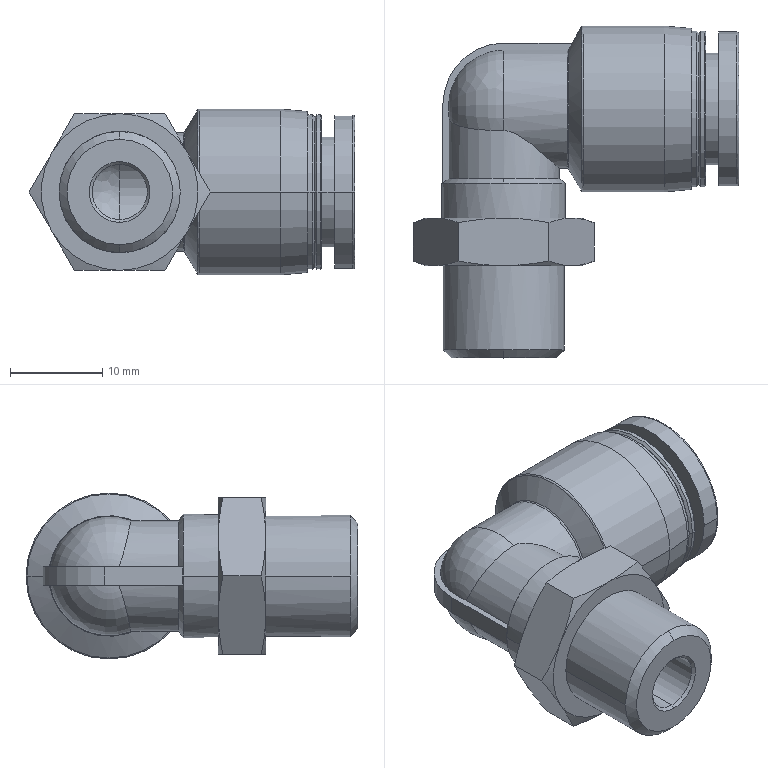Part | STEP file | PL1002 | 1 solid | 88 faces | box 35.315 x 36 x 18 mm | volume 6237 mm3 | cone 28 | cylinder 27 | plane 19 | spline 12 | other 2 | commonest cylinder face diameters 8 x4 16.9 x4 13.4 x3 6 x2 10 x2 12 x2